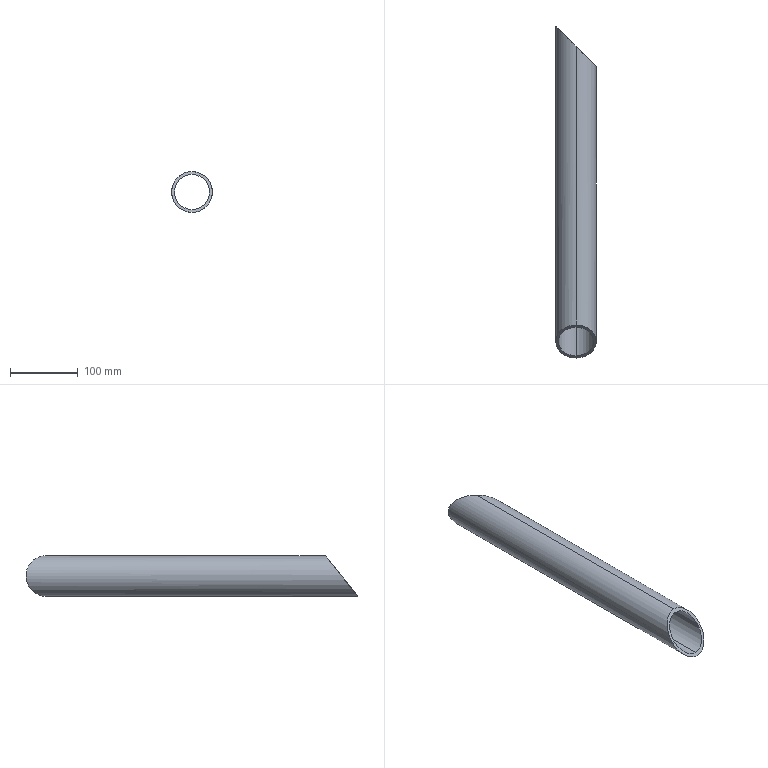Part | SolidWorks | features ICE 2, Extrusion 1 | 1 solid | 6 faces | box 60 x 490 x 60 mm | volume 306614 mm3 | cylinder 4 | plane 2 | commonest cylinder face diameters 52 x2 60 x2
STEP:
#1=CARTESIAN_POINT('',(0.,460.,-26.));
#2=VERTEX_POINT('',#1);
#3=CARTESIAN_POINT('',(0.,460.,26.));
#4=VERTEX_POINT('',#3);
#5=CARTESIAN_POINT('',(0.,460.,-26.));
#6=CARTESIAN_POINT('',(-52.,512.,-26.));
#7=CARTESIAN_POINT('',(-52.,512.,26.));
#8=CARTESIAN_POINT('',(0.,460.,26.));
#9=(BOUNDED_CURVE()B_SPLINE_CURVE(3,(#5,#6,#7,#8),.UNSPECIFIED.,.F.,.F.)B_SPLINE_CURVE_WITH_KNOTS((4,4),(1.571,4.712),.UNSPECIFIED.)CURVE()GEOMETRIC_REPRESENTATION_ITEM()RATIONAL_B_SPLINE_CURVE((1.,0.3333,0.3333,1.))REPRESENTATION_ITEM(''));
#10=EDGE_CURVE('',#2,#4,#9,.T.);
#11=ORIENTED_EDGE('',*,*,#10,.T.);
#12=CARTESIAN_POINT('',(0.,45.348,26.));
#13=VERTEX_POINT('',#12);
#14=CARTESIAN_POINT('',(0.,490.,26.));
#15=DIRECTION('',(0.,-1.,0.));
#16=VECTOR('',#15,1000.);
#17=LINE('',#14,#16);
#18=EDGE_CURVE('',#4,#13,#17,.T.);
#19=ORIENTED_EDGE('',*,*,#18,.T.);
#20=CARTESIAN_POINT('',(0.,3.239,-26.));
#21=VERTEX_POINT('',#20);
#22=CARTESIAN_POINT('',(0.,45.348,26.));
#23=CARTESIAN_POINT('',(-52.,45.348,26.));
#24=CARTESIAN_POINT('',(-52.,3.239,-26.));
#25=CARTESIAN_POINT('',(0.,3.239,-26.));
#26=(BOUNDED_CURVE()B_SPLINE_CURVE(3,(#22,#23,#24,#25),.UNSPECIFIED.,.F.,.F.)B_SPLINE_CURVE_WITH_KNOTS((4,4),(3.142,6.283),.UNSPECIFIED.)CURVE()GEOMETRIC_REPRESENTATION_ITEM()RATIONAL_B_SPLINE_CURVE((1.,0.3333,0.3333,1.))REPRESENTATION_ITEM(''));
#27=EDGE_CURVE('',#13,#21,#26,.T.);
#28=ORIENTED_EDGE('',*,*,#27,.T.);
#29=CARTESIAN_POINT('',(0.,490.,-26.));
#30=DIRECTION('',(0.,-1.,0.));
#31=VECTOR('',#30,1000.);
#32=LINE('',#29,#31);
#33=EDGE_CURVE('',#2,#21,#32,.T.);
#34=ORIENTED_EDGE('',*,*,#33,.F.);
#35=EDGE_LOOP('',(#11,#19,#28,#34));
#36=FACE_OUTER_BOUND('',#35,.T.);
#37=CARTESIAN_POINT('',(0.,490.,0.));
#38=DIRECTION('',(0.,-1.,0.));
#39=DIRECTION('',(0.,0.,-1.));
#40=AXIS2_PLACEMENT_3D('',#37,#38,#39);
#41=CYLINDRICAL_SURFACE('',#40,26.);
#42=ADVANCED_FACE('',(#36),#41,.F.);
#43=CARTESIAN_POINT('',(0.,460.,30.));
#44=VERTEX_POINT('',#43);
#45=CARTESIAN_POINT('',(0.,460.,-30.));
#46=VERTEX_POINT('',#45);
#47=CARTESIAN_POINT('',(0.,460.,30.));
#48=CARTESIAN_POINT('',(60.,400.,30.));
#49=CARTESIAN_POINT('',(60.,400.,-30.));
#50=CARTESIAN_POINT('',(0.,460.,-30.));
#51=(BOUNDED_CURVE()B_SPLINE_CURVE(3,(#47,#48,#49,#50),.UNSPECIFIED.,.F.,.F.)B_SPLINE_CURVE_WITH_KNOTS((4,4),(4.712,7.854),.UNSPECIFIED.)CURVE()GEOMETRIC_REPRESENTATION_ITEM()RATIONAL_B_SPLINE_CURVE((1.,0.3333,0.3333,1.))REPRESENTATION_ITEM(''));
#52=EDGE_CURVE('',#44,#46,#51,.T.);
#53=ORIENTED_EDGE('',*,*,#52,.F.);
#54=CARTESIAN_POINT('',(0.,48.587,30.));
#55=VERTEX_POINT('',#54);
#56=CARTESIAN_POINT('',(0.,490.,30.));
#57=DIRECTION('',(0.,-1.,0.));
#58=VECTOR('',#57,1000.);
#59=LINE('',#56,#58);
#60=EDGE_CURVE('',#44,#55,#59,.T.);
#61=ORIENTED_EDGE('',*,*,#60,.T.);
#62=CARTESIAN_POINT('',(0.,0.,-30.));
#63=VERTEX_POINT('',#62);
#64=CARTESIAN_POINT('',(0.,0.,-30.));
#65=CARTESIAN_POINT('',(60.,0.,-30.));
#66=CARTESIAN_POINT('',(60.,48.587,30.));
#67=CARTESIAN_POINT('',(0.,48.587,30.));
#68=(BOUNDED_CURVE()B_SPLINE_CURVE(3,(#64,#65,#66,#67),.UNSPECIFIED.,.F.,.T.)B_SPLINE_CURVE_WITH_KNOTS((4,4),(0.,3.142),.UNSPECIFIED.)CURVE()GEOMETRIC_REPRESENTATION_ITEM()RATIONAL_B_SPLINE_CURVE((1.,0.3333,0.3333,1.))REPRESENTATION_ITEM(''));
#69=EDGE_CURVE('',#63,#55,#68,.T.);
#70=ORIENTED_EDGE('',*,*,#69,.F.);
#71=CARTESIAN_POINT('',(0.,490.,-30.));
#72=DIRECTION('',(0.,-1.,0.));
#73=VECTOR('',#72,1000.);
#74=LINE('',#71,#73);
#75=EDGE_CURVE('',#46,#63,#74,.T.);
#76=ORIENTED_EDGE('',*,*,#75,.F.);
#77=EDGE_LOOP('',(#53,#61,#70,#76));
#78=FACE_OUTER_BOUND('',#77,.T.);
#79=CARTESIAN_POINT('',(0.,490.,0.));
#80=DIRECTION('',(0.,-1.,0.));
#81=DIRECTION('',(0.,0.,-1.));
#82=AXIS2_PLACEMENT_3D('',#79,#80,#81);
#83=CYLINDRICAL_SURFACE('',#82,30.);
#84=ADVANCED_FACE('',(#78),#83,.T.);
#85=ORIENTED_EDGE('',*,*,#60,.F.);
#86=CARTESIAN_POINT('',(0.,460.,-30.));
#87=CARTESIAN_POINT('',(-60.,520.,-30.));
#88=CARTESIAN_POINT('',(-60.,520.,30.));
#89=CARTESIAN_POINT('',(0.,460.,30.));
#90=(BOUNDED_CURVE()B_SPLINE_CURVE(3,(#86,#87,#88,#89),.UNSPECIFIED.,.F.,.T.)B_SPLINE_CURVE_WITH_KNOTS((4,4),(1.571,4.712),.UNSPECIFIED.)CURVE()GEOMETRIC_REPRESENTATION_ITEM()RATIONAL_B_SPLINE_CURVE((1.,0.3333,0.3333,1.))REPRESENTATION_ITEM(''));
#91=EDGE_CURVE('',#46,#44,#90,.T.);
#92=ORIENTED_EDGE('',*,*,#91,.F.);
#93=ORIENTED_EDGE('',*,*,#75,.T.);
#94=CARTESIAN_POINT('',(0.,48.587,30.));
#95=CARTESIAN_POINT('',(-60.,48.587,30.));
#96=CARTESIAN_POINT('',(-60.,0.,-30.));
#97=CARTESIAN_POINT('',(0.,0.,-30.));
#98=(BOUNDED_CURVE()B_SPLINE_CURVE(3,(#94,#95,#96,#97),.UNSPECIFIED.,.F.,.F.)B_SPLINE_CURVE_WITH_KNOTS((4,4),(3.142,6.283),.UNSPECIFIED.)CURVE()GEOMETRIC_REPRESENTATION_ITEM()RATIONAL_B_SPLINE_CURVE((1.,0.3333,0.3333,1.))REPRESENTATION_ITEM(''));
#99=EDGE_CURVE('',#55,#63,#98,.T.);
#100=ORIENTED_EDGE('',*,*,#99,.F.);
#101=EDGE_LOOP('',(#85,#92,#93,#100));
#102=FACE_OUTER_BOUND('',#101,.T.);
#103=CARTESIAN_POINT('',(0.,490.,0.));
#104=DIRECTION('',(0.,-1.,0.));
#105=DIRECTION('',(0.,0.,-1.));
#106=AXIS2_PLACEMENT_3D('',#103,#104,#105);
#107=CYLINDRICAL_SURFACE('',#106,30.);
#108=ADVANCED_FACE('',(#102),#107,.T.);
#109=ORIENTED_EDGE('',*,*,#18,.F.);
#110=CARTESIAN_POINT('',(0.,460.,26.));
#111=CARTESIAN_POINT('',(52.,408.,26.));
#112=CARTESIAN_POINT('',(52.,408.,-26.));
#113=CARTESIAN_POINT('',(0.,460.,-26.));
#114=(BOUNDED_CURVE()B_SPLINE_CURVE(3,(#110,#111,#112,#113),.UNSPECIFIED.,.F.,.T.)B_SPLINE_CURVE_WITH_KNOTS((4,4),(4.712,7.854),.UNSPECIFIED.)CURVE()GEOMETRIC_REPRESENTATION_ITEM()RATIONAL_B_SPLINE_CURVE((1.,0.3333,0.3333,1.))REPRESENTATION_ITEM(''));
#115=EDGE_CURVE('',#4,#2,#114,.T.);
#116=ORIENTED_EDGE('',*,*,#115,.T.);
#117=ORIENTED_EDGE('',*,*,#33,.T.);
#118=CARTESIAN_POINT('',(0.,3.239,-26.));
#119=CARTESIAN_POINT('',(52.,3.239,-26.));
#120=CARTESIAN_POINT('',(52.,45.348,26.));
#121=CARTESIAN_POINT('',(0.,45.348,26.));
#122=(BOUNDED_CURVE()B_SPLINE_CURVE(3,(#118,#119,#120,#121),.UNSPECIFIED.,.F.,.F.)B_SPLINE_CURVE_WITH_KNOTS((4,4),(0.,3.142),.UNSPECIFIED.)CURVE()GEOMETRIC_REPRESENTATION_ITEM()RATIONAL_B_SPLINE_CURVE((1.,0.3333,0.3333,1.))REPRESENTATION_ITEM(''));
#123=EDGE_CURVE('',#21,#13,#122,.T.);
#124=ORIENTED_EDGE('',*,*,#123,.T.);
#125=EDGE_LOOP('',(#109,#116,#117,#124));
#126=FACE_OUTER_BOUND('',#125,.T.);
#127=CARTESIAN_POINT('',(0.,490.,0.));
#128=DIRECTION('',(0.,-1.,0.));
#129=DIRECTION('',(0.,0.,-1.));
#130=AXIS2_PLACEMENT_3D('',#127,#128,#129);
#131=CYLINDRICAL_SURFACE('',#130,26.);
#132=ADVANCED_FACE('',(#126),#131,.F.);
#133=ORIENTED_EDGE('',*,*,#10,.F.);
#134=ORIENTED_EDGE('',*,*,#115,.F.);
#135=EDGE_LOOP('',(#133,#134));
#136=FACE_BOUND('',#135,.T.);
#137=ORIENTED_EDGE('',*,*,#91,.T.);
#138=ORIENTED_EDGE('',*,*,#52,.T.);
#139=EDGE_LOOP('',(#137,#138));
#140=FACE_OUTER_BOUND('',#139,.T.);
#141=CARTESIAN_POINT('',(-30.,490.,659.116));
#142=DIRECTION('',(0.7071,0.7071,0.));
#143=DIRECTION('',(-0.7071,0.7071,0.));
#144=AXIS2_PLACEMENT_3D('',#141,#142,#143);
#145=PLANE('',#144);
#146=ADVANCED_FACE('',(#136,#140),#145,.T.);
#147=ORIENTED_EDGE('',*,*,#123,.F.);
#148=ORIENTED_EDGE('',*,*,#27,.F.);
#149=EDGE_LOOP('',(#147,#148));
#150=FACE_BOUND('',#149,.T.);
#151=ORIENTED_EDGE('',*,*,#69,.T.);
#152=ORIENTED_EDGE('',*,*,#99,.T.);
#153=EDGE_LOOP('',(#151,#152));
#154=FACE_OUTER_BOUND('',#153,.T.);
#155=CARTESIAN_POINT('',(621.616,0.,-30.));
#156=DIRECTION('',(0.,-0.7771,0.6293));
#157=DIRECTION('',(0.,-0.6293,-0.7771));
#158=AXIS2_PLACEMENT_3D('',#155,#156,#157);
#159=PLANE('',#158);
#160=ADVANCED_FACE('',(#150,#154),#159,.T.);
#161=CLOSED_SHELL('',(#42,#84,#108,#132,#146,#160));
#162=MANIFOLD_SOLID_BREP('',#161);
#163=CARTESIAN_POINT('',(0.,0.,0.));
#164=DIRECTION('',(0.,0.,1.));
#165=DIRECTION('',(1.,0.,0.));
#166=AXIS2_PLACEMENT_3D('',#163,#164,#165);
#167=(LENGTH_UNIT()NAMED_UNIT(*)SI_UNIT(.MILLI.,.METRE.));
#168=UNCERTAINTY_MEASURE_WITH_UNIT(LENGTH_MEASURE(0.00001),#167,'','');
#169=(NAMED_UNIT(*)PLANE_ANGLE_UNIT()SI_UNIT($,.RADIAN.));
#170=(NAMED_UNIT(*)SI_UNIT($,.STERADIAN.)SOLID_ANGLE_UNIT());
#171=(GEOMETRIC_REPRESENTATION_CONTEXT(3)GLOBAL_UNCERTAINTY_ASSIGNED_CONTEXT((#168))GLOBAL_UNIT_ASSIGNED_CONTEXT((#167,#169,#170))REPRESENTATION_CONTEXT('',''));
#172=ADVANCED_BREP_SHAPE_REPRESENTATION('',(#162,#166),#171);